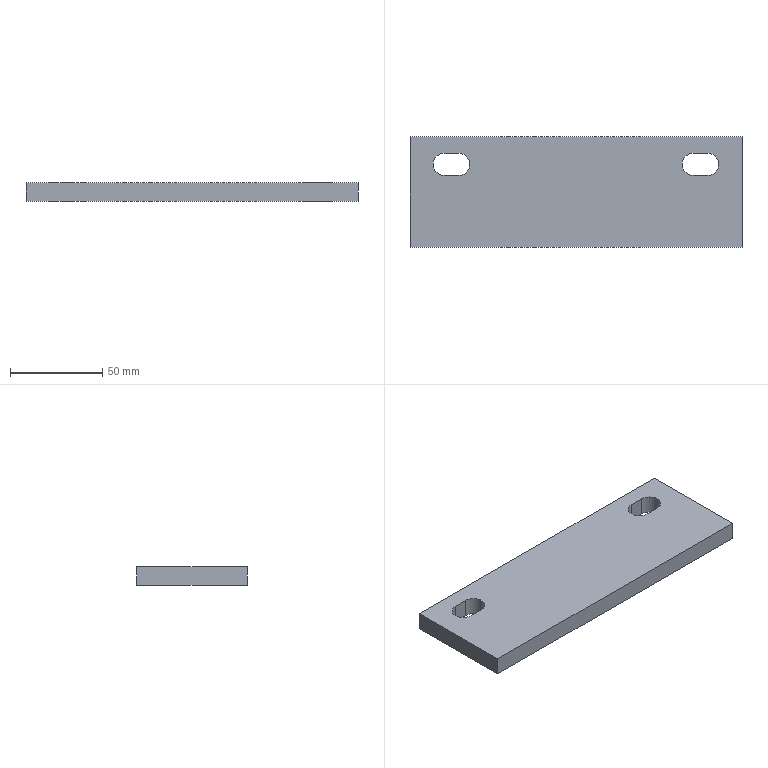Part | SolidWorks | features Extrusion 1 | 1 solid | 16 faces | box 180 x 60 x 10 mm | volume 103818 mm3 | plane 10 | cylinder 6 | commonest cylinder face diameters 12 x6
STEP:
#1=CARTESIAN_POINT('',(63.5,21.,10.));
#2=VERTEX_POINT('',#1);
#3=CARTESIAN_POINT('',(57.5,15.,10.));
#4=VERTEX_POINT('',#3);
#5=CARTESIAN_POINT('',(63.5,15.,10.));
#6=DIRECTION('',(0.,0.,1.));
#7=DIRECTION('',(-1.,0.,0.));
#8=AXIS2_PLACEMENT_3D('',#5,#6,#7);
#9=CIRCLE('',#8,6.);
#10=EDGE_CURVE('',#2,#4,#9,.T.);
#11=ORIENTED_EDGE('',*,*,#10,.T.);
#12=CARTESIAN_POINT('',(57.5,15.,0.));
#13=VERTEX_POINT('',#12);
#14=CARTESIAN_POINT('',(57.5,15.,10.));
#15=DIRECTION('',(0.,0.,-1.));
#16=VECTOR('',#15,1000.);
#17=LINE('',#14,#16);
#18=EDGE_CURVE('',#4,#13,#17,.T.);
#19=ORIENTED_EDGE('',*,*,#18,.T.);
#20=CARTESIAN_POINT('',(63.5,21.,0.));
#21=VERTEX_POINT('',#20);
#22=CARTESIAN_POINT('',(63.5,15.,0.));
#23=DIRECTION('',(0.,0.,1.));
#24=DIRECTION('',(-1.,0.,0.));
#25=AXIS2_PLACEMENT_3D('',#22,#23,#24);
#26=CIRCLE('',#25,6.);
#27=EDGE_CURVE('',#21,#13,#26,.T.);
#28=ORIENTED_EDGE('',*,*,#27,.F.);
#29=CARTESIAN_POINT('',(63.5,21.,10.));
#30=DIRECTION('',(0.,0.,-1.));
#31=VECTOR('',#30,1000.);
#32=LINE('',#29,#31);
#33=EDGE_CURVE('',#2,#21,#32,.T.);
#34=ORIENTED_EDGE('',*,*,#33,.F.);
#35=EDGE_LOOP('',(#11,#19,#28,#34));
#36=FACE_OUTER_BOUND('',#35,.T.);
#37=CARTESIAN_POINT('',(63.5,15.,10.));
#38=DIRECTION('',(0.,0.,-1.));
#39=DIRECTION('',(-1.,0.,0.));
#40=AXIS2_PLACEMENT_3D('',#37,#38,#39);
#41=CYLINDRICAL_SURFACE('',#40,6.);
#42=ADVANCED_FACE('',(#36),#41,.F.);
#43=CARTESIAN_POINT('',(-71.5,21.,10.));
#44=VERTEX_POINT('',#43);
#45=CARTESIAN_POINT('',(-77.5,15.,10.));
#46=VERTEX_POINT('',#45);
#47=CARTESIAN_POINT('',(-71.5,15.,10.));
#48=DIRECTION('',(0.,0.,1.));
#49=DIRECTION('',(-1.,0.,0.));
#50=AXIS2_PLACEMENT_3D('',#47,#48,#49);
#51=CIRCLE('',#50,6.);
#52=EDGE_CURVE('',#44,#46,#51,.T.);
#53=ORIENTED_EDGE('',*,*,#52,.T.);
#54=CARTESIAN_POINT('',(-77.5,15.,0.));
#55=VERTEX_POINT('',#54);
#56=CARTESIAN_POINT('',(-77.5,15.,10.));
#57=DIRECTION('',(0.,0.,-1.));
#58=VECTOR('',#57,1000.);
#59=LINE('',#56,#58);
#60=EDGE_CURVE('',#46,#55,#59,.T.);
#61=ORIENTED_EDGE('',*,*,#60,.T.);
#62=CARTESIAN_POINT('',(-71.5,21.,0.));
#63=VERTEX_POINT('',#62);
#64=CARTESIAN_POINT('',(-71.5,15.,0.));
#65=DIRECTION('',(0.,0.,1.));
#66=DIRECTION('',(-1.,0.,0.));
#67=AXIS2_PLACEMENT_3D('',#64,#65,#66);
#68=CIRCLE('',#67,6.);
#69=EDGE_CURVE('',#63,#55,#68,.T.);
#70=ORIENTED_EDGE('',*,*,#69,.F.);
#71=CARTESIAN_POINT('',(-71.5,21.,10.));
#72=DIRECTION('',(0.,0.,-1.));
#73=VECTOR('',#72,1000.);
#74=LINE('',#71,#73);
#75=EDGE_CURVE('',#44,#63,#74,.T.);
#76=ORIENTED_EDGE('',*,*,#75,.F.);
#77=EDGE_LOOP('',(#53,#61,#70,#76));
#78=FACE_OUTER_BOUND('',#77,.T.);
#79=CARTESIAN_POINT('',(-71.5,15.,10.));
#80=DIRECTION('',(0.,0.,-1.));
#81=DIRECTION('',(-1.,0.,0.));
#82=AXIS2_PLACEMENT_3D('',#79,#80,#81);
#83=CYLINDRICAL_SURFACE('',#82,6.);
#84=ADVANCED_FACE('',(#78),#83,.F.);
#85=CARTESIAN_POINT('',(90.,-30.,10.));
#86=VERTEX_POINT('',#85);
#87=CARTESIAN_POINT('',(90.,30.,10.));
#88=VERTEX_POINT('',#87);
#89=CARTESIAN_POINT('',(90.,30.,10.));
#90=DIRECTION('',(0.,1.,0.));
#91=VECTOR('',#90,1000.);
#92=LINE('',#89,#91);
#93=EDGE_CURVE('',#86,#88,#92,.T.);
#94=ORIENTED_EDGE('',*,*,#93,.T.);
#95=CARTESIAN_POINT('',(-90.,30.,10.));
#96=VERTEX_POINT('',#95);
#97=CARTESIAN_POINT('',(-90.,30.,10.));
#98=DIRECTION('',(-1.,0.,0.));
#99=VECTOR('',#98,1000.);
#100=LINE('',#97,#99);
#101=EDGE_CURVE('',#88,#96,#100,.T.);
#102=ORIENTED_EDGE('',*,*,#101,.T.);
#103=CARTESIAN_POINT('',(-90.,-30.,10.));
#104=VERTEX_POINT('',#103);
#105=CARTESIAN_POINT('',(-90.,30.,10.));
#106=DIRECTION('',(0.,-1.,0.));
#107=VECTOR('',#106,1000.);
#108=LINE('',#105,#107);
#109=EDGE_CURVE('',#96,#104,#108,.T.);
#110=ORIENTED_EDGE('',*,*,#109,.T.);
#111=CARTESIAN_POINT('',(-90.,-30.,10.));
#112=DIRECTION('',(1.,0.,0.));
#113=VECTOR('',#112,1000.);
#114=LINE('',#111,#113);
#115=EDGE_CURVE('',#104,#86,#114,.T.);
#116=ORIENTED_EDGE('',*,*,#115,.T.);
#117=EDGE_LOOP('',(#94,#102,#110,#116));
#118=FACE_OUTER_BOUND('',#117,.T.);
#119=CARTESIAN_POINT('',(-63.5,21.,10.));
#120=VERTEX_POINT('',#119);
#121=CARTESIAN_POINT('',(-71.5,21.,10.));
#122=DIRECTION('',(-1.,0.,0.));
#123=VECTOR('',#122,1000.);
#124=LINE('',#121,#123);
#125=EDGE_CURVE('',#120,#44,#124,.T.);
#126=ORIENTED_EDGE('',*,*,#125,.F.);
#127=CARTESIAN_POINT('',(-63.5,9.,10.));
#128=VERTEX_POINT('',#127);
#129=CARTESIAN_POINT('',(-63.5,15.,10.));
#130=DIRECTION('',(0.,0.,1.));
#131=DIRECTION('',(-1.,0.,0.));
#132=AXIS2_PLACEMENT_3D('',#129,#130,#131);
#133=CIRCLE('',#132,6.);
#134=EDGE_CURVE('',#128,#120,#133,.T.);
#135=ORIENTED_EDGE('',*,*,#134,.F.);
#136=CARTESIAN_POINT('',(-71.5,9.,10.));
#137=VERTEX_POINT('',#136);
#138=CARTESIAN_POINT('',(-71.5,9.,10.));
#139=DIRECTION('',(1.,0.,0.));
#140=VECTOR('',#139,1000.);
#141=LINE('',#138,#140);
#142=EDGE_CURVE('',#137,#128,#141,.T.);
#143=ORIENTED_EDGE('',*,*,#142,.F.);
#144=CARTESIAN_POINT('',(-71.5,15.,10.));
#145=DIRECTION('',(0.,0.,1.));
#146=DIRECTION('',(-1.,0.,0.));
#147=AXIS2_PLACEMENT_3D('',#144,#145,#146);
#148=CIRCLE('',#147,6.);
#149=EDGE_CURVE('',#46,#137,#148,.T.);
#150=ORIENTED_EDGE('',*,*,#149,.F.);
#151=ORIENTED_EDGE('',*,*,#52,.F.);
#152=EDGE_LOOP('',(#126,#135,#143,#150,#151));
#153=FACE_BOUND('',#152,.T.);
#154=CARTESIAN_POINT('',(71.5,21.,10.));
#155=VERTEX_POINT('',#154);
#156=CARTESIAN_POINT('',(63.5,21.,10.));
#157=DIRECTION('',(-1.,0.,0.));
#158=VECTOR('',#157,1000.);
#159=LINE('',#156,#158);
#160=EDGE_CURVE('',#155,#2,#159,.T.);
#161=ORIENTED_EDGE('',*,*,#160,.F.);
#162=CARTESIAN_POINT('',(71.5,9.,10.));
#163=VERTEX_POINT('',#162);
#164=CARTESIAN_POINT('',(71.5,15.,10.));
#165=DIRECTION('',(0.,0.,1.));
#166=DIRECTION('',(-1.,0.,0.));
#167=AXIS2_PLACEMENT_3D('',#164,#165,#166);
#168=CIRCLE('',#167,6.);
#169=EDGE_CURVE('',#163,#155,#168,.T.);
#170=ORIENTED_EDGE('',*,*,#169,.F.);
#171=CARTESIAN_POINT('',(63.5,9.,10.));
#172=VERTEX_POINT('',#171);
#173=CARTESIAN_POINT('',(63.5,9.,10.));
#174=DIRECTION('',(1.,0.,0.));
#175=VECTOR('',#174,1000.);
#176=LINE('',#173,#175);
#177=EDGE_CURVE('',#172,#163,#176,.T.);
#178=ORIENTED_EDGE('',*,*,#177,.F.);
#179=CARTESIAN_POINT('',(63.5,15.,10.));
#180=DIRECTION('',(0.,0.,1.));
#181=DIRECTION('',(-1.,0.,0.));
#182=AXIS2_PLACEMENT_3D('',#179,#180,#181);
#183=CIRCLE('',#182,6.);
#184=EDGE_CURVE('',#4,#172,#183,.T.);
#185=ORIENTED_EDGE('',*,*,#184,.F.);
#186=ORIENTED_EDGE('',*,*,#10,.F.);
#187=EDGE_LOOP('',(#161,#170,#178,#185,#186));
#188=FACE_BOUND('',#187,.T.);
#189=CARTESIAN_POINT('',(0.,0.,10.));
#190=DIRECTION('',(0.,0.,1.));
#191=DIRECTION('',(1.,0.,0.));
#192=AXIS2_PLACEMENT_3D('',#189,#190,#191);
#193=PLANE('',#192);
#194=ADVANCED_FACE('',(#118,#153,#188),#193,.T.);
#195=CARTESIAN_POINT('',(-63.5,9.,0.));
#196=VERTEX_POINT('',#195);
#197=CARTESIAN_POINT('',(-63.5,21.,0.));
#198=VERTEX_POINT('',#197);
#199=CARTESIAN_POINT('',(-63.5,15.,0.));
#200=DIRECTION('',(0.,0.,1.));
#201=DIRECTION('',(-1.,0.,0.));
#202=AXIS2_PLACEMENT_3D('',#199,#200,#201);
#203=CIRCLE('',#202,6.);
#204=EDGE_CURVE('',#196,#198,#203,.T.);
#205=ORIENTED_EDGE('',*,*,#204,.T.);
#206=CARTESIAN_POINT('',(-71.5,21.,0.));
#207=DIRECTION('',(-1.,0.,0.));
#208=VECTOR('',#207,1000.);
#209=LINE('',#206,#208);
#210=EDGE_CURVE('',#198,#63,#209,.T.);
#211=ORIENTED_EDGE('',*,*,#210,.T.);
#212=ORIENTED_EDGE('',*,*,#69,.T.);
#213=CARTESIAN_POINT('',(-71.5,9.,0.));
#214=VERTEX_POINT('',#213);
#215=CARTESIAN_POINT('',(-71.5,15.,0.));
#216=DIRECTION('',(0.,0.,1.));
#217=DIRECTION('',(-1.,0.,0.));
#218=AXIS2_PLACEMENT_3D('',#215,#216,#217);
#219=CIRCLE('',#218,6.);
#220=EDGE_CURVE('',#55,#214,#219,.T.);
#221=ORIENTED_EDGE('',*,*,#220,.T.);
#222=CARTESIAN_POINT('',(-71.5,9.,0.));
#223=DIRECTION('',(1.,0.,0.));
#224=VECTOR('',#223,1000.);
#225=LINE('',#222,#224);
#226=EDGE_CURVE('',#214,#196,#225,.T.);
#227=ORIENTED_EDGE('',*,*,#226,.T.);
#228=EDGE_LOOP('',(#205,#211,#212,#221,#227));
#229=FACE_BOUND('',#228,.T.);
#230=CARTESIAN_POINT('',(90.,-30.,0.));
#231=VERTEX_POINT('',#230);
#232=CARTESIAN_POINT('',(90.,30.,0.));
#233=VERTEX_POINT('',#232);
#234=CARTESIAN_POINT('',(90.,30.,0.));
#235=DIRECTION('',(0.,1.,0.));
#236=VECTOR('',#235,1000.);
#237=LINE('',#234,#236);
#238=EDGE_CURVE('',#231,#233,#237,.T.);
#239=ORIENTED_EDGE('',*,*,#238,.F.);
#240=CARTESIAN_POINT('',(-90.,-30.,0.));
#241=VERTEX_POINT('',#240);
#242=CARTESIAN_POINT('',(-90.,-30.,0.));
#243=DIRECTION('',(1.,0.,0.));
#244=VECTOR('',#243,1000.);
#245=LINE('',#242,#244);
#246=EDGE_CURVE('',#241,#231,#245,.T.);
#247=ORIENTED_EDGE('',*,*,#246,.F.);
#248=CARTESIAN_POINT('',(-90.,30.,0.));
#249=VERTEX_POINT('',#248);
#250=CARTESIAN_POINT('',(-90.,30.,0.));
#251=DIRECTION('',(0.,-1.,0.));
#252=VECTOR('',#251,1000.);
#253=LINE('',#250,#252);
#254=EDGE_CURVE('',#249,#241,#253,.T.);
#255=ORIENTED_EDGE('',*,*,#254,.F.);
#256=CARTESIAN_POINT('',(-90.,30.,0.));
#257=DIRECTION('',(-1.,0.,0.));
#258=VECTOR('',#257,1000.);
#259=LINE('',#256,#258);
#260=EDGE_CURVE('',#233,#249,#259,.T.);
#261=ORIENTED_EDGE('',*,*,#260,.F.);
#262=EDGE_LOOP('',(#239,#247,#255,#261));
#263=FACE_OUTER_BOUND('',#262,.T.);
#264=CARTESIAN_POINT('',(71.5,9.,0.));
#265=VERTEX_POINT('',#264);
#266=CARTESIAN_POINT('',(71.5,21.,0.));
#267=VERTEX_POINT('',#266);
#268=CARTESIAN_POINT('',(71.5,15.,0.));
#269=DIRECTION('',(0.,0.,1.));
#270=DIRECTION('',(-1.,0.,0.));
#271=AXIS2_PLACEMENT_3D('',#268,#269,#270);
#272=CIRCLE('',#271,6.);
#273=EDGE_CURVE('',#265,#267,#272,.T.);
#274=ORIENTED_EDGE('',*,*,#273,.T.);
#275=CARTESIAN_POINT('',(63.5,21.,0.));
#276=DIRECTION('',(-1.,0.,0.));
#277=VECTOR('',#276,1000.);
#278=LINE('',#275,#277);
#279=EDGE_CURVE('',#267,#21,#278,.T.);
#280=ORIENTED_EDGE('',*,*,#279,.T.);
#281=ORIENTED_EDGE('',*,*,#27,.T.);
#282=CARTESIAN_POINT('',(63.5,9.,0.));
#283=VERTEX_POINT('',#282);
#284=CARTESIAN_POINT('',(63.5,15.,0.));
#285=DIRECTION('',(0.,0.,1.));
#286=DIRECTION('',(-1.,0.,0.));
#287=AXIS2_PLACEMENT_3D('',#284,#285,#286);
#288=CIRCLE('',#287,6.);
#289=EDGE_CURVE('',#13,#283,#288,.T.);
#290=ORIENTED_EDGE('',*,*,#289,.T.);
#291=CARTESIAN_POINT('',(63.5,9.,0.));
#292=DIRECTION('',(1.,0.,0.));
#293=VECTOR('',#292,1000.);
#294=LINE('',#291,#293);
#295=EDGE_CURVE('',#283,#265,#294,.T.);
#296=ORIENTED_EDGE('',*,*,#295,.T.);
#297=EDGE_LOOP('',(#274,#280,#281,#290,#296));
#298=FACE_BOUND('',#297,.T.);
#299=CARTESIAN_POINT('',(0.,0.,0.));
#300=DIRECTION('',(0.,0.,1.));
#301=DIRECTION('',(1.,0.,0.));
#302=AXIS2_PLACEMENT_3D('',#299,#300,#301);
#303=PLANE('',#302);
#304=ADVANCED_FACE('',(#229,#263,#298),#303,.F.);
#305=ORIENTED_EDGE('',*,*,#238,.T.);
#306=CARTESIAN_POINT('',(90.,30.,10.));
#307=DIRECTION('',(0.,0.,-1.));
#308=VECTOR('',#307,1000.);
#309=LINE('',#306,#308);
#310=EDGE_CURVE('',#88,#233,#309,.T.);
#311=ORIENTED_EDGE('',*,*,#310,.F.);
#312=ORIENTED_EDGE('',*,*,#93,.F.);
#313=CARTESIAN_POINT('',(90.,-30.,10.));
#314=DIRECTION('',(0.,0.,-1.));
#315=VECTOR('',#314,1000.);
#316=LINE('',#313,#315);
#317=EDGE_CURVE('',#86,#231,#316,.T.);
#318=ORIENTED_EDGE('',*,*,#317,.T.);
#319=EDGE_LOOP('',(#305,#311,#312,#318));
#320=FACE_OUTER_BOUND('',#319,.T.);
#321=CARTESIAN_POINT('',(90.,30.,10.));
#322=DIRECTION('',(-1.,0.,0.));
#323=DIRECTION('',(0.,-1.,0.));
#324=AXIS2_PLACEMENT_3D('',#321,#322,#323);
#325=PLANE('',#324);
#326=ADVANCED_FACE('',(#320),#325,.F.);
#327=ORIENTED_EDGE('',*,*,#260,.T.);
#328=CARTESIAN_POINT('',(-90.,30.,10.));
#329=DIRECTION('',(0.,0.,-1.));
#330=VECTOR('',#329,1000.);
#331=LINE('',#328,#330);
#332=EDGE_CURVE('',#96,#249,#331,.T.);
#333=ORIENTED_EDGE('',*,*,#332,.F.);
#334=ORIENTED_EDGE('',*,*,#101,.F.);
#335=ORIENTED_EDGE('',*,*,#310,.T.);
#336=EDGE_LOOP('',(#327,#333,#334,#335));
#337=FACE_OUTER_BOUND('',#336,.T.);
#338=CARTESIAN_POINT('',(-90.,30.,10.));
#339=DIRECTION('',(0.,-1.,0.));
#340=DIRECTION('',(0.,0.,-1.));
#341=AXIS2_PLACEMENT_3D('',#338,#339,#340);
#342=PLANE('',#341);
#343=ADVANCED_FACE('',(#337),#342,.F.);
#344=ORIENTED_EDGE('',*,*,#254,.T.);
#345=CARTESIAN_POINT('',(-90.,-30.,10.));
#346=DIRECTION('',(0.,0.,-1.));
#347=VECTOR('',#346,1000.);
#348=LINE('',#345,#347);
#349=EDGE_CURVE('',#104,#241,#348,.T.);
#350=ORIENTED_EDGE('',*,*,#349,.F.);
#351=ORIENTED_EDGE('',*,*,#109,.F.);
#352=ORIENTED_EDGE('',*,*,#332,.T.);
#353=EDGE_LOOP('',(#344,#350,#351,#352));
#354=FACE_OUTER_BOUND('',#353,.T.);
#355=CARTESIAN_POINT('',(-90.,30.,10.));
#356=DIRECTION('',(1.,0.,0.));
#357=DIRECTION('',(0.,1.,0.));
#358=AXIS2_PLACEMENT_3D('',#355,#356,#357);
#359=PLANE('',#358);
#360=ADVANCED_FACE('',(#354),#359,.F.);
#361=ORIENTED_EDGE('',*,*,#246,.T.);
#362=ORIENTED_EDGE('',*,*,#317,.F.);
#363=ORIENTED_EDGE('',*,*,#115,.F.);
#364=ORIENTED_EDGE('',*,*,#349,.T.);
#365=EDGE_LOOP('',(#361,#362,#363,#364));
#366=FACE_OUTER_BOUND('',#365,.T.);
#367=CARTESIAN_POINT('',(-90.,-30.,10.));
#368=DIRECTION('',(0.,1.,0.));
#369=DIRECTION('',(0.,0.,1.));
#370=AXIS2_PLACEMENT_3D('',#367,#368,#369);
#371=PLANE('',#370);
#372=ADVANCED_FACE('',(#366),#371,.F.);
#373=ORIENTED_EDGE('',*,*,#204,.F.);
#374=CARTESIAN_POINT('',(-63.5,9.,10.));
#375=DIRECTION('',(0.,0.,-1.));
#376=VECTOR('',#375,1000.);
#377=LINE('',#374,#376);
#378=EDGE_CURVE('',#128,#196,#377,.T.);
#379=ORIENTED_EDGE('',*,*,#378,.F.);
#380=ORIENTED_EDGE('',*,*,#134,.T.);
#381=CARTESIAN_POINT('',(-63.5,21.,10.));
#382=DIRECTION('',(0.,0.,-1.));
#383=VECTOR('',#382,1000.);
#384=LINE('',#381,#383);
#385=EDGE_CURVE('',#120,#198,#384,.T.);
#386=ORIENTED_EDGE('',*,*,#385,.T.);
#387=EDGE_LOOP('',(#373,#379,#380,#386));
#388=FACE_OUTER_BOUND('',#387,.T.);
#389=CARTESIAN_POINT('',(-63.5,15.,10.));
#390=DIRECTION('',(0.,0.,-1.));
#391=DIRECTION('',(-1.,0.,0.));
#392=AXIS2_PLACEMENT_3D('',#389,#390,#391);
#393=CYLINDRICAL_SURFACE('',#392,6.);
#394=ADVANCED_FACE('',(#388),#393,.F.);
#395=ORIENTED_EDGE('',*,*,#210,.F.);
#396=ORIENTED_EDGE('',*,*,#385,.F.);
#397=ORIENTED_EDGE('',*,*,#125,.T.);
#398=ORIENTED_EDGE('',*,*,#75,.T.);
#399=EDGE_LOOP('',(#395,#396,#397,#398));
#400=FACE_OUTER_BOUND('',#399,.T.);
#401=CARTESIAN_POINT('',(-71.5,21.,10.));
#402=DIRECTION('',(0.,-1.,0.));
#403=DIRECTION('',(0.,0.,-1.));
#404=AXIS2_PLACEMENT_3D('',#401,#402,#403);
#405=PLANE('',#404);
#406=ADVANCED_FACE('',(#400),#405,.T.);
#407=ORIENTED_EDGE('',*,*,#60,.F.);
#408=ORIENTED_EDGE('',*,*,#149,.T.);
#409=CARTESIAN_POINT('',(-71.5,9.,10.));
#410=DIRECTION('',(0.,0.,-1.));
#411=VECTOR('',#410,1000.);
#412=LINE('',#409,#411);
#413=EDGE_CURVE('',#137,#214,#412,.T.);
#414=ORIENTED_EDGE('',*,*,#413,.T.);
#415=ORIENTED_EDGE('',*,*,#220,.F.);
#416=EDGE_LOOP('',(#407,#408,#414,#415));
#417=FACE_OUTER_BOUND('',#416,.T.);
#418=CARTESIAN_POINT('',(-71.5,15.,10.));
#419=DIRECTION('',(0.,0.,-1.));
#420=DIRECTION('',(-1.,0.,0.));
#421=AXIS2_PLACEMENT_3D('',#418,#419,#420);
#422=CYLINDRICAL_SURFACE('',#421,6.);
#423=ADVANCED_FACE('',(#417),#422,.F.);
#424=ORIENTED_EDGE('',*,*,#226,.F.);
#425=ORIENTED_EDGE('',*,*,#413,.F.);
#426=ORIENTED_EDGE('',*,*,#142,.T.);
#427=ORIENTED_EDGE('',*,*,#378,.T.);
#428=EDGE_LOOP('',(#424,#425,#426,#427));
#429=FACE_OUTER_BOUND('',#428,.T.);
#430=CARTESIAN_POINT('',(-71.5,9.,10.));
#431=DIRECTION('',(0.,1.,0.));
#432=DIRECTION('',(0.,0.,1.));
#433=AXIS2_PLACEMENT_3D('',#430,#431,#432);
#434=PLANE('',#433);
#435=ADVANCED_FACE('',(#429),#434,.T.);
#436=ORIENTED_EDGE('',*,*,#273,.F.);
#437=CARTESIAN_POINT('',(71.5,9.,10.));
#438=DIRECTION('',(0.,0.,-1.));
#439=VECTOR('',#438,1000.);
#440=LINE('',#437,#439);
#441=EDGE_CURVE('',#163,#265,#440,.T.);
#442=ORIENTED_EDGE('',*,*,#441,.F.);
#443=ORIENTED_EDGE('',*,*,#169,.T.);
#444=CARTESIAN_POINT('',(71.5,21.,10.));
#445=DIRECTION('',(0.,0.,-1.));
#446=VECTOR('',#445,1000.);
#447=LINE('',#444,#446);
#448=EDGE_CURVE('',#155,#267,#447,.T.);
#449=ORIENTED_EDGE('',*,*,#448,.T.);
#450=EDGE_LOOP('',(#436,#442,#443,#449));
#451=FACE_OUTER_BOUND('',#450,.T.);
#452=CARTESIAN_POINT('',(71.5,15.,10.));
#453=DIRECTION('',(0.,0.,-1.));
#454=DIRECTION('',(-1.,0.,0.));
#455=AXIS2_PLACEMENT_3D('',#452,#453,#454);
#456=CYLINDRICAL_SURFACE('',#455,6.);
#457=ADVANCED_FACE('',(#451),#456,.F.);
#458=ORIENTED_EDGE('',*,*,#279,.F.);
#459=ORIENTED_EDGE('',*,*,#448,.F.);
#460=ORIENTED_EDGE('',*,*,#160,.T.);
#461=ORIENTED_EDGE('',*,*,#33,.T.);
#462=EDGE_LOOP('',(#458,#459,#460,#461));
#463=FACE_OUTER_BOUND('',#462,.T.);
#464=CARTESIAN_POINT('',(63.5,21.,10.));
#465=DIRECTION('',(0.,-1.,0.));
#466=DIRECTION('',(0.,0.,-1.));
#467=AXIS2_PLACEMENT_3D('',#464,#465,#466);
#468=PLANE('',#467);
#469=ADVANCED_FACE('',(#463),#468,.T.);
#470=ORIENTED_EDGE('',*,*,#18,.F.);
#471=ORIENTED_EDGE('',*,*,#184,.T.);
#472=CARTESIAN_POINT('',(63.5,9.,10.));
#473=DIRECTION('',(0.,0.,-1.));
#474=VECTOR('',#473,1000.);
#475=LINE('',#472,#474);
#476=EDGE_CURVE('',#172,#283,#475,.T.);
#477=ORIENTED_EDGE('',*,*,#476,.T.);
#478=ORIENTED_EDGE('',*,*,#289,.F.);
#479=EDGE_LOOP('',(#470,#471,#477,#478));
#480=FACE_OUTER_BOUND('',#479,.T.);
#481=CARTESIAN_POINT('',(63.5,15.,10.));
#482=DIRECTION('',(0.,0.,-1.));
#483=DIRECTION('',(-1.,0.,0.));
#484=AXIS2_PLACEMENT_3D('',#481,#482,#483);
#485=CYLINDRICAL_SURFACE('',#484,6.);
#486=ADVANCED_FACE('',(#480),#485,.F.);
#487=ORIENTED_EDGE('',*,*,#295,.F.);
#488=ORIENTED_EDGE('',*,*,#476,.F.);
#489=ORIENTED_EDGE('',*,*,#177,.T.);
#490=ORIENTED_EDGE('',*,*,#441,.T.);
#491=EDGE_LOOP('',(#487,#488,#489,#490));
#492=FACE_OUTER_BOUND('',#491,.T.);
#493=CARTESIAN_POINT('',(63.5,9.,10.));
#494=DIRECTION('',(0.,1.,0.));
#495=DIRECTION('',(0.,0.,1.));
#496=AXIS2_PLACEMENT_3D('',#493,#494,#495);
#497=PLANE('',#496);
#498=ADVANCED_FACE('',(#492),#497,.T.);
#499=CLOSED_SHELL('',(#42,#84,#194,#304,#326,#343,#360,#372,#394,#406,#423,#435,#457,#469,#486,#498));
#500=MANIFOLD_SOLID_BREP('',#499);
#501=CARTESIAN_POINT('',(0.,0.,0.));
#502=DIRECTION('',(0.,0.,1.));
#503=DIRECTION('',(1.,0.,0.));
#504=AXIS2_PLACEMENT_3D('',#501,#502,#503);
#505=(LENGTH_UNIT()NAMED_UNIT(*)SI_UNIT(.MILLI.,.METRE.));
#506=UNCERTAINTY_MEASURE_WITH_UNIT(LENGTH_MEASURE(0.00001),#505,'','');
#507=(NAMED_UNIT(*)PLANE_ANGLE_UNIT()SI_UNIT($,.RADIAN.));
#508=(NAMED_UNIT(*)SI_UNIT($,.STERADIAN.)SOLID_ANGLE_UNIT());
#509=(GEOMETRIC_REPRESENTATION_CONTEXT(3)GLOBAL_UNCERTAINTY_ASSIGNED_CONTEXT((#506))GLOBAL_UNIT_ASSIGNED_CONTEXT((#505,#507,#508))REPRESENTATION_CONTEXT('',''));
#510=ADVANCED_BREP_SHAPE_REPRESENTATION('',(#500,#504),#509);